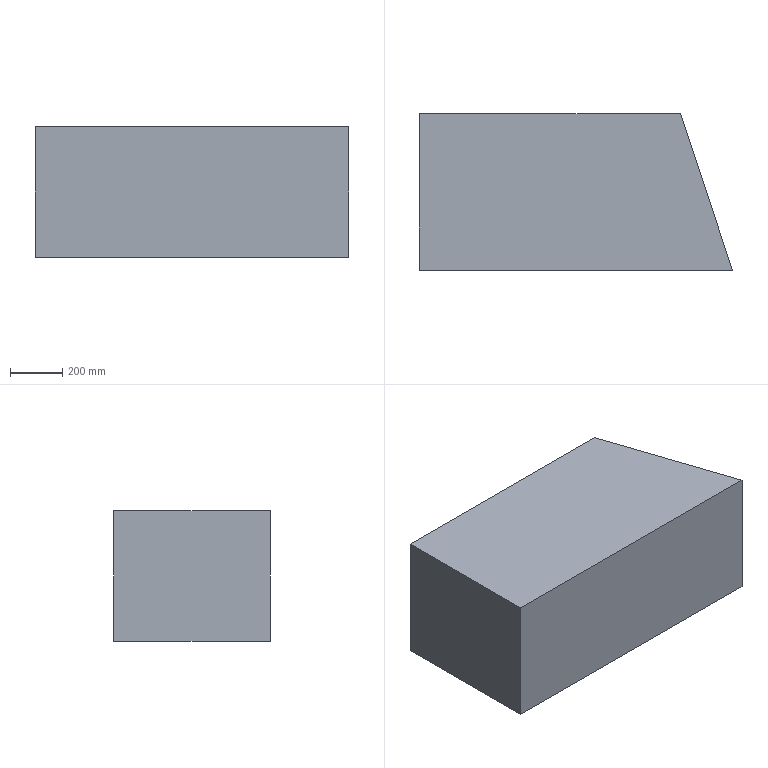Part | SolidWorks | features Extrusion 1 | 1 solid | 6 faces | box 1200 x 600 x 500 mm | volume 330000000 mm3 | plane 6
STEP:
#1=CARTESIAN_POINT('',(0.,0.,0.));
#2=VERTEX_POINT('',#1);
#3=CARTESIAN_POINT('',(1200.,0.,0.));
#4=VERTEX_POINT('',#3);
#5=CARTESIAN_POINT('',(1200.,0.,0.));
#6=DIRECTION('',(1.,0.,0.));
#7=VECTOR('',#6,1000.);
#8=LINE('',#5,#7);
#9=EDGE_CURVE('',#2,#4,#8,.T.);
#10=ORIENTED_EDGE('',*,*,#9,.T.);
#11=CARTESIAN_POINT('',(1200.,0.,500.));
#12=VERTEX_POINT('',#11);
#13=CARTESIAN_POINT('',(1200.,0.,500.));
#14=DIRECTION('',(0.,0.,-1.));
#15=VECTOR('',#14,1000.);
#16=LINE('',#13,#15);
#17=EDGE_CURVE('',#12,#4,#16,.T.);
#18=ORIENTED_EDGE('',*,*,#17,.F.);
#19=CARTESIAN_POINT('',(0.,0.,500.));
#20=VERTEX_POINT('',#19);
#21=CARTESIAN_POINT('',(1200.,0.,500.));
#22=DIRECTION('',(1.,0.,0.));
#23=VECTOR('',#22,1000.);
#24=LINE('',#21,#23);
#25=EDGE_CURVE('',#20,#12,#24,.T.);
#26=ORIENTED_EDGE('',*,*,#25,.F.);
#27=CARTESIAN_POINT('',(0.,0.,500.));
#28=DIRECTION('',(0.,0.,-1.));
#29=VECTOR('',#28,1000.);
#30=LINE('',#27,#29);
#31=EDGE_CURVE('',#20,#2,#30,.T.);
#32=ORIENTED_EDGE('',*,*,#31,.T.);
#33=EDGE_LOOP('',(#10,#18,#26,#32));
#34=FACE_OUTER_BOUND('',#33,.T.);
#35=CARTESIAN_POINT('',(1200.,0.,500.));
#36=DIRECTION('',(0.,1.,0.));
#37=DIRECTION('',(-1.,0.,0.));
#38=AXIS2_PLACEMENT_3D('',#35,#36,#37);
#39=PLANE('',#38);
#40=ADVANCED_FACE('',(#34),#39,.F.);
#41=CARTESIAN_POINT('',(1000.,600.,0.));
#42=VERTEX_POINT('',#41);
#43=CARTESIAN_POINT('',(1000.,600.,0.));
#44=DIRECTION('',(-0.3162,0.9487,0.));
#45=VECTOR('',#44,1000.);
#46=LINE('',#43,#45);
#47=EDGE_CURVE('',#4,#42,#46,.T.);
#48=ORIENTED_EDGE('',*,*,#47,.T.);
#49=CARTESIAN_POINT('',(1000.,600.,500.));
#50=VERTEX_POINT('',#49);
#51=CARTESIAN_POINT('',(1000.,600.,500.));
#52=DIRECTION('',(0.,0.,-1.));
#53=VECTOR('',#52,1000.);
#54=LINE('',#51,#53);
#55=EDGE_CURVE('',#50,#42,#54,.T.);
#56=ORIENTED_EDGE('',*,*,#55,.F.);
#57=CARTESIAN_POINT('',(1000.,600.,500.));
#58=DIRECTION('',(-0.3162,0.9487,0.));
#59=VECTOR('',#58,1000.);
#60=LINE('',#57,#59);
#61=EDGE_CURVE('',#12,#50,#60,.T.);
#62=ORIENTED_EDGE('',*,*,#61,.F.);
#63=ORIENTED_EDGE('',*,*,#17,.T.);
#64=EDGE_LOOP('',(#48,#56,#62,#63));
#65=FACE_OUTER_BOUND('',#64,.T.);
#66=CARTESIAN_POINT('',(1000.,600.,500.));
#67=DIRECTION('',(-0.9487,-0.3162,0.));
#68=DIRECTION('',(0.3162,-0.9487,0.));
#69=AXIS2_PLACEMENT_3D('',#66,#67,#68);
#70=PLANE('',#69);
#71=ADVANCED_FACE('',(#65),#70,.F.);
#72=CARTESIAN_POINT('',(0.,600.,0.));
#73=VERTEX_POINT('',#72);
#74=CARTESIAN_POINT('',(0.,600.,0.));
#75=DIRECTION('',(-1.,0.,0.));
#76=VECTOR('',#75,1000.);
#77=LINE('',#74,#76);
#78=EDGE_CURVE('',#42,#73,#77,.T.);
#79=ORIENTED_EDGE('',*,*,#78,.T.);
#80=CARTESIAN_POINT('',(0.,600.,500.));
#81=VERTEX_POINT('',#80);
#82=CARTESIAN_POINT('',(0.,600.,500.));
#83=DIRECTION('',(0.,0.,-1.));
#84=VECTOR('',#83,1000.);
#85=LINE('',#82,#84);
#86=EDGE_CURVE('',#81,#73,#85,.T.);
#87=ORIENTED_EDGE('',*,*,#86,.F.);
#88=CARTESIAN_POINT('',(0.,600.,500.));
#89=DIRECTION('',(-1.,0.,0.));
#90=VECTOR('',#89,1000.);
#91=LINE('',#88,#90);
#92=EDGE_CURVE('',#50,#81,#91,.T.);
#93=ORIENTED_EDGE('',*,*,#92,.F.);
#94=ORIENTED_EDGE('',*,*,#55,.T.);
#95=EDGE_LOOP('',(#79,#87,#93,#94));
#96=FACE_OUTER_BOUND('',#95,.T.);
#97=CARTESIAN_POINT('',(0.,600.,500.));
#98=DIRECTION('',(0.,-1.,0.));
#99=DIRECTION('',(0.,0.,-1.));
#100=AXIS2_PLACEMENT_3D('',#97,#98,#99);
#101=PLANE('',#100);
#102=ADVANCED_FACE('',(#96),#101,.F.);
#103=CARTESIAN_POINT('',(0.,0.,0.));
#104=DIRECTION('',(0.,-1.,0.));
#105=VECTOR('',#104,1000.);
#106=LINE('',#103,#105);
#107=EDGE_CURVE('',#73,#2,#106,.T.);
#108=ORIENTED_EDGE('',*,*,#107,.T.);
#109=ORIENTED_EDGE('',*,*,#31,.F.);
#110=CARTESIAN_POINT('',(0.,0.,500.));
#111=DIRECTION('',(0.,-1.,0.));
#112=VECTOR('',#111,1000.);
#113=LINE('',#110,#112);
#114=EDGE_CURVE('',#81,#20,#113,.T.);
#115=ORIENTED_EDGE('',*,*,#114,.F.);
#116=ORIENTED_EDGE('',*,*,#86,.T.);
#117=EDGE_LOOP('',(#108,#109,#115,#116));
#118=FACE_OUTER_BOUND('',#117,.T.);
#119=CARTESIAN_POINT('',(0.,0.,500.));
#120=DIRECTION('',(1.,0.,0.));
#121=DIRECTION('',(0.,0.,-1.));
#122=AXIS2_PLACEMENT_3D('',#119,#120,#121);
#123=PLANE('',#122);
#124=ADVANCED_FACE('',(#118),#123,.F.);
#125=ORIENTED_EDGE('',*,*,#25,.T.);
#126=ORIENTED_EDGE('',*,*,#61,.T.);
#127=ORIENTED_EDGE('',*,*,#92,.T.);
#128=ORIENTED_EDGE('',*,*,#114,.T.);
#129=EDGE_LOOP('',(#125,#126,#127,#128));
#130=FACE_OUTER_BOUND('',#129,.T.);
#131=CARTESIAN_POINT('',(0.,0.,500.));
#132=DIRECTION('',(0.,0.,-1.));
#133=DIRECTION('',(-1.,0.,0.));
#134=AXIS2_PLACEMENT_3D('',#131,#132,#133);
#135=PLANE('',#134);
#136=ADVANCED_FACE('',(#130),#135,.F.);
#137=ORIENTED_EDGE('',*,*,#9,.F.);
#138=ORIENTED_EDGE('',*,*,#107,.F.);
#139=ORIENTED_EDGE('',*,*,#78,.F.);
#140=ORIENTED_EDGE('',*,*,#47,.F.);
#141=EDGE_LOOP('',(#137,#138,#139,#140));
#142=FACE_OUTER_BOUND('',#141,.T.);
#143=CARTESIAN_POINT('',(0.,0.,0.));
#144=DIRECTION('',(0.,0.,-1.));
#145=DIRECTION('',(-1.,0.,0.));
#146=AXIS2_PLACEMENT_3D('',#143,#144,#145);
#147=PLANE('',#146);
#148=ADVANCED_FACE('',(#142),#147,.T.);
#149=CLOSED_SHELL('',(#40,#71,#102,#124,#136,#148));
#150=MANIFOLD_SOLID_BREP('',#149);
#151=CARTESIAN_POINT('',(0.,0.,0.));
#152=DIRECTION('',(0.,0.,1.));
#153=DIRECTION('',(1.,0.,0.));
#154=AXIS2_PLACEMENT_3D('',#151,#152,#153);
#155=(LENGTH_UNIT()NAMED_UNIT(*)SI_UNIT(.MILLI.,.METRE.));
#156=UNCERTAINTY_MEASURE_WITH_UNIT(LENGTH_MEASURE(0.00001),#155,'','');
#157=(NAMED_UNIT(*)PLANE_ANGLE_UNIT()SI_UNIT($,.RADIAN.));
#158=(NAMED_UNIT(*)SI_UNIT($,.STERADIAN.)SOLID_ANGLE_UNIT());
#159=(GEOMETRIC_REPRESENTATION_CONTEXT(3)GLOBAL_UNCERTAINTY_ASSIGNED_CONTEXT((#156))GLOBAL_UNIT_ASSIGNED_CONTEXT((#155,#157,#158))REPRESENTATION_CONTEXT('',''));
#160=ADVANCED_BREP_SHAPE_REPRESENTATION('',(#150,#154),#159);